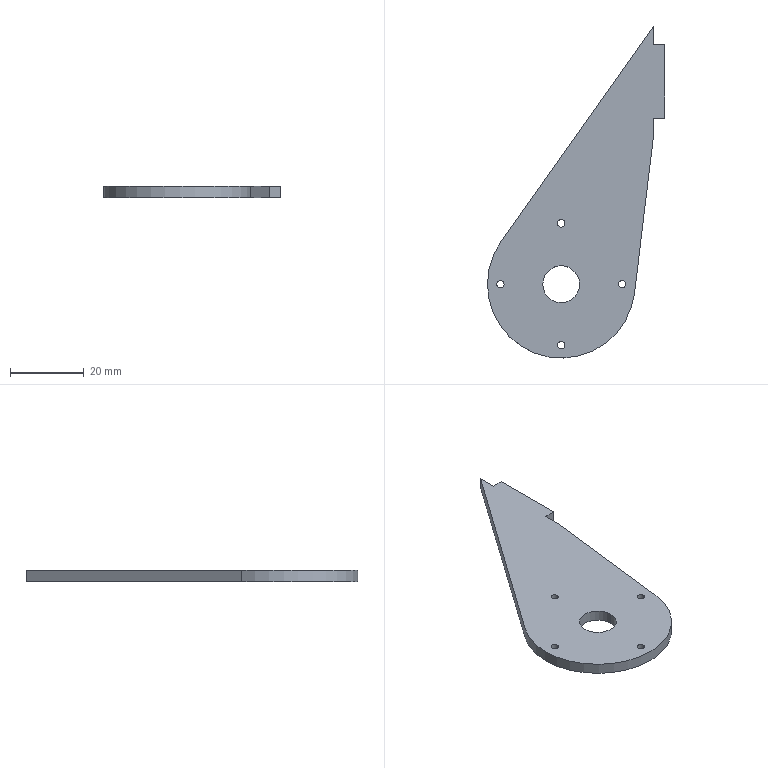Part | SolidWorks | features ICE 3, Extrusion 1 | 1 solid | 20 faces | box 48 x 90 x 3 mm | volume 6643 mm3 | cylinder 11 | plane 9 | commonest cylinder face diameters 2 x8 10 x2 40 x1
STEP:
#1=CARTESIAN_POINT('',(-17.5,0.,-3.));
#2=VERTEX_POINT('',#1);
#3=CARTESIAN_POINT('',(-15.5,0.,-3.));
#4=VERTEX_POINT('',#3);
#5=CARTESIAN_POINT('',(-16.5,0.,-3.));
#6=DIRECTION('',(0.,0.,1.));
#7=DIRECTION('',(1.,0.,0.));
#8=AXIS2_PLACEMENT_3D('',#5,#6,#7);
#9=CIRCLE('',#8,1.);
#10=EDGE_CURVE('',#2,#4,#9,.T.);
#11=ORIENTED_EDGE('',*,*,#10,.F.);
#12=CARTESIAN_POINT('',(-17.5,0.,0.));
#13=VERTEX_POINT('',#12);
#14=CARTESIAN_POINT('',(-17.5,0.,-10.));
#15=DIRECTION('',(0.,0.,1.));
#16=VECTOR('',#15,1000.);
#17=LINE('',#14,#16);
#18=EDGE_CURVE('',#2,#13,#17,.T.);
#19=ORIENTED_EDGE('',*,*,#18,.T.);
#20=CARTESIAN_POINT('',(-15.5,0.,0.));
#21=VERTEX_POINT('',#20);
#22=CARTESIAN_POINT('',(-16.5,0.,0.));
#23=DIRECTION('',(0.,0.,1.));
#24=DIRECTION('',(1.,0.,0.));
#25=AXIS2_PLACEMENT_3D('',#22,#23,#24);
#26=CIRCLE('',#25,1.);
#27=EDGE_CURVE('',#13,#21,#26,.T.);
#28=ORIENTED_EDGE('',*,*,#27,.T.);
#29=CARTESIAN_POINT('',(-15.5,0.,-10.));
#30=DIRECTION('',(0.,0.,1.));
#31=VECTOR('',#30,1000.);
#32=LINE('',#29,#31);
#33=EDGE_CURVE('',#4,#21,#32,.T.);
#34=ORIENTED_EDGE('',*,*,#33,.F.);
#35=EDGE_LOOP('',(#11,#19,#28,#34));
#36=FACE_OUTER_BOUND('',#35,.T.);
#37=CARTESIAN_POINT('',(-16.5,0.,-10.));
#38=DIRECTION('',(0.,0.,1.));
#39=DIRECTION('',(1.,0.,0.));
#40=AXIS2_PLACEMENT_3D('',#37,#38,#39);
#41=CYLINDRICAL_SURFACE('',#40,1.);
#42=ADVANCED_FACE('',(#36),#41,.F.);
#43=CARTESIAN_POINT('',(15.5,0.,-3.));
#44=VERTEX_POINT('',#43);
#45=CARTESIAN_POINT('',(17.5,0.,-3.));
#46=VERTEX_POINT('',#45);
#47=CARTESIAN_POINT('',(16.5,0.,-3.));
#48=DIRECTION('',(0.,0.,1.));
#49=DIRECTION('',(1.,0.,0.));
#50=AXIS2_PLACEMENT_3D('',#47,#48,#49);
#51=CIRCLE('',#50,1.);
#52=EDGE_CURVE('',#44,#46,#51,.T.);
#53=ORIENTED_EDGE('',*,*,#52,.F.);
#54=CARTESIAN_POINT('',(15.5,0.,0.));
#55=VERTEX_POINT('',#54);
#56=CARTESIAN_POINT('',(15.5,0.,-10.));
#57=DIRECTION('',(0.,0.,1.));
#58=VECTOR('',#57,1000.);
#59=LINE('',#56,#58);
#60=EDGE_CURVE('',#44,#55,#59,.T.);
#61=ORIENTED_EDGE('',*,*,#60,.T.);
#62=CARTESIAN_POINT('',(17.5,0.,0.));
#63=VERTEX_POINT('',#62);
#64=CARTESIAN_POINT('',(16.5,0.,0.));
#65=DIRECTION('',(0.,0.,1.));
#66=DIRECTION('',(1.,0.,0.));
#67=AXIS2_PLACEMENT_3D('',#64,#65,#66);
#68=CIRCLE('',#67,1.);
#69=EDGE_CURVE('',#55,#63,#68,.T.);
#70=ORIENTED_EDGE('',*,*,#69,.T.);
#71=CARTESIAN_POINT('',(17.5,0.,-10.));
#72=DIRECTION('',(0.,0.,1.));
#73=VECTOR('',#72,1000.);
#74=LINE('',#71,#73);
#75=EDGE_CURVE('',#46,#63,#74,.T.);
#76=ORIENTED_EDGE('',*,*,#75,.F.);
#77=EDGE_LOOP('',(#53,#61,#70,#76));
#78=FACE_OUTER_BOUND('',#77,.T.);
#79=CARTESIAN_POINT('',(16.5,0.,-10.));
#80=DIRECTION('',(0.,0.,1.));
#81=DIRECTION('',(1.,0.,0.));
#82=AXIS2_PLACEMENT_3D('',#79,#80,#81);
#83=CYLINDRICAL_SURFACE('',#82,1.);
#84=ADVANCED_FACE('',(#78),#83,.F.);
#85=CARTESIAN_POINT('',(-1.,-16.5,-3.));
#86=VERTEX_POINT('',#85);
#87=CARTESIAN_POINT('',(1.,-16.5,-3.));
#88=VERTEX_POINT('',#87);
#89=CARTESIAN_POINT('',(0.,-16.5,-3.));
#90=DIRECTION('',(0.,0.,1.));
#91=DIRECTION('',(1.,0.,0.));
#92=AXIS2_PLACEMENT_3D('',#89,#90,#91);
#93=CIRCLE('',#92,1.);
#94=EDGE_CURVE('',#86,#88,#93,.T.);
#95=ORIENTED_EDGE('',*,*,#94,.F.);
#96=CARTESIAN_POINT('',(-1.,-16.5,0.));
#97=VERTEX_POINT('',#96);
#98=CARTESIAN_POINT('',(-1.,-16.5,-10.));
#99=DIRECTION('',(0.,0.,1.));
#100=VECTOR('',#99,1000.);
#101=LINE('',#98,#100);
#102=EDGE_CURVE('',#86,#97,#101,.T.);
#103=ORIENTED_EDGE('',*,*,#102,.T.);
#104=CARTESIAN_POINT('',(1.,-16.5,0.));
#105=VERTEX_POINT('',#104);
#106=CARTESIAN_POINT('',(0.,-16.5,0.));
#107=DIRECTION('',(0.,0.,1.));
#108=DIRECTION('',(1.,0.,0.));
#109=AXIS2_PLACEMENT_3D('',#106,#107,#108);
#110=CIRCLE('',#109,1.);
#111=EDGE_CURVE('',#97,#105,#110,.T.);
#112=ORIENTED_EDGE('',*,*,#111,.T.);
#113=CARTESIAN_POINT('',(1.,-16.5,-10.));
#114=DIRECTION('',(0.,0.,1.));
#115=VECTOR('',#114,1000.);
#116=LINE('',#113,#115);
#117=EDGE_CURVE('',#88,#105,#116,.T.);
#118=ORIENTED_EDGE('',*,*,#117,.F.);
#119=EDGE_LOOP('',(#95,#103,#112,#118));
#120=FACE_OUTER_BOUND('',#119,.T.);
#121=CARTESIAN_POINT('',(0.,-16.5,-10.));
#122=DIRECTION('',(0.,0.,1.));
#123=DIRECTION('',(1.,0.,0.));
#124=AXIS2_PLACEMENT_3D('',#121,#122,#123);
#125=CYLINDRICAL_SURFACE('',#124,1.);
#126=ADVANCED_FACE('',(#120),#125,.F.);
#127=CARTESIAN_POINT('',(-1.,16.5,-3.));
#128=VERTEX_POINT('',#127);
#129=CARTESIAN_POINT('',(1.,16.5,-3.));
#130=VERTEX_POINT('',#129);
#131=CARTESIAN_POINT('',(0.,16.5,-3.));
#132=DIRECTION('',(0.,0.,1.));
#133=DIRECTION('',(1.,0.,0.));
#134=AXIS2_PLACEMENT_3D('',#131,#132,#133);
#135=CIRCLE('',#134,1.);
#136=EDGE_CURVE('',#128,#130,#135,.T.);
#137=ORIENTED_EDGE('',*,*,#136,.F.);
#138=CARTESIAN_POINT('',(-1.,16.5,0.));
#139=VERTEX_POINT('',#138);
#140=CARTESIAN_POINT('',(-1.,16.5,-10.));
#141=DIRECTION('',(0.,0.,1.));
#142=VECTOR('',#141,1000.);
#143=LINE('',#140,#142);
#144=EDGE_CURVE('',#128,#139,#143,.T.);
#145=ORIENTED_EDGE('',*,*,#144,.T.);
#146=CARTESIAN_POINT('',(1.,16.5,0.));
#147=VERTEX_POINT('',#146);
#148=CARTESIAN_POINT('',(0.,16.5,0.));
#149=DIRECTION('',(0.,0.,1.));
#150=DIRECTION('',(1.,0.,0.));
#151=AXIS2_PLACEMENT_3D('',#148,#149,#150);
#152=CIRCLE('',#151,1.);
#153=EDGE_CURVE('',#139,#147,#152,.T.);
#154=ORIENTED_EDGE('',*,*,#153,.T.);
#155=CARTESIAN_POINT('',(1.,16.5,-10.));
#156=DIRECTION('',(0.,0.,1.));
#157=VECTOR('',#156,1000.);
#158=LINE('',#155,#157);
#159=EDGE_CURVE('',#130,#147,#158,.T.);
#160=ORIENTED_EDGE('',*,*,#159,.F.);
#161=EDGE_LOOP('',(#137,#145,#154,#160));
#162=FACE_OUTER_BOUND('',#161,.T.);
#163=CARTESIAN_POINT('',(0.,16.5,-10.));
#164=DIRECTION('',(0.,0.,1.));
#165=DIRECTION('',(1.,0.,0.));
#166=AXIS2_PLACEMENT_3D('',#163,#164,#165);
#167=CYLINDRICAL_SURFACE('',#166,1.);
#168=ADVANCED_FACE('',(#162),#167,.F.);
#169=CARTESIAN_POINT('',(-5.,0.,-3.));
#170=VERTEX_POINT('',#169);
#171=CARTESIAN_POINT('',(5.,0.,-3.));
#172=VERTEX_POINT('',#171);
#173=CARTESIAN_POINT('',(0.,0.,-3.));
#174=DIRECTION('',(0.,0.,1.));
#175=DIRECTION('',(1.,0.,0.));
#176=AXIS2_PLACEMENT_3D('',#173,#174,#175);
#177=CIRCLE('',#176,5.);
#178=EDGE_CURVE('',#170,#172,#177,.T.);
#179=ORIENTED_EDGE('',*,*,#178,.F.);
#180=CARTESIAN_POINT('',(-5.,0.,0.));
#181=VERTEX_POINT('',#180);
#182=CARTESIAN_POINT('',(-5.,0.,-10.));
#183=DIRECTION('',(0.,0.,1.));
#184=VECTOR('',#183,1000.);
#185=LINE('',#182,#184);
#186=EDGE_CURVE('',#170,#181,#185,.T.);
#187=ORIENTED_EDGE('',*,*,#186,.T.);
#188=CARTESIAN_POINT('',(5.,0.,0.));
#189=VERTEX_POINT('',#188);
#190=CARTESIAN_POINT('',(0.,0.,0.));
#191=DIRECTION('',(0.,0.,1.));
#192=DIRECTION('',(1.,0.,0.));
#193=AXIS2_PLACEMENT_3D('',#190,#191,#192);
#194=CIRCLE('',#193,5.);
#195=EDGE_CURVE('',#181,#189,#194,.T.);
#196=ORIENTED_EDGE('',*,*,#195,.T.);
#197=CARTESIAN_POINT('',(5.,0.,-10.));
#198=DIRECTION('',(0.,0.,1.));
#199=VECTOR('',#198,1000.);
#200=LINE('',#197,#199);
#201=EDGE_CURVE('',#172,#189,#200,.T.);
#202=ORIENTED_EDGE('',*,*,#201,.F.);
#203=EDGE_LOOP('',(#179,#187,#196,#202));
#204=FACE_OUTER_BOUND('',#203,.T.);
#205=CARTESIAN_POINT('',(0.,0.,-10.));
#206=DIRECTION('',(0.,0.,1.));
#207=DIRECTION('',(1.,0.,0.));
#208=AXIS2_PLACEMENT_3D('',#205,#206,#207);
#209=CYLINDRICAL_SURFACE('',#208,5.);
#210=ADVANCED_FACE('',(#204),#209,.F.);
#211=CARTESIAN_POINT('',(25.,65.,-3.));
#212=VERTEX_POINT('',#211);
#213=CARTESIAN_POINT('',(25.,65.,0.));
#214=VERTEX_POINT('',#213);
#215=CARTESIAN_POINT('',(25.,65.,0.));
#216=DIRECTION('',(0.,0.,1.));
#217=VECTOR('',#216,1000.);
#218=LINE('',#215,#217);
#219=EDGE_CURVE('',#212,#214,#218,.T.);
#220=ORIENTED_EDGE('',*,*,#219,.F.);
#221=CARTESIAN_POINT('',(25.,70.,-3.));
#222=VERTEX_POINT('',#221);
#223=CARTESIAN_POINT('',(25.,70.,-3.));
#224=DIRECTION('',(0.,1.,0.));
#225=VECTOR('',#224,1000.);
#226=LINE('',#223,#225);
#227=EDGE_CURVE('',#212,#222,#226,.T.);
#228=ORIENTED_EDGE('',*,*,#227,.T.);
#229=CARTESIAN_POINT('',(25.,70.,0.));
#230=VERTEX_POINT('',#229);
#231=CARTESIAN_POINT('',(25.,70.,-3.));
#232=DIRECTION('',(0.,0.,1.));
#233=VECTOR('',#232,1000.);
#234=LINE('',#231,#233);
#235=EDGE_CURVE('',#222,#230,#234,.T.);
#236=ORIENTED_EDGE('',*,*,#235,.T.);
#237=CARTESIAN_POINT('',(25.,70.,0.));
#238=DIRECTION('',(0.,1.,0.));
#239=VECTOR('',#238,1000.);
#240=LINE('',#237,#239);
#241=EDGE_CURVE('',#214,#230,#240,.T.);
#242=ORIENTED_EDGE('',*,*,#241,.F.);
#243=EDGE_LOOP('',(#220,#228,#236,#242));
#244=FACE_OUTER_BOUND('',#243,.T.);
#245=CARTESIAN_POINT('',(25.,70.,-3.));
#246=DIRECTION('',(1.,0.,0.));
#247=DIRECTION('',(0.,1.,0.));
#248=AXIS2_PLACEMENT_3D('',#245,#246,#247);
#249=PLANE('',#248);
#250=ADVANCED_FACE('',(#244),#249,.T.);
#251=CARTESIAN_POINT('',(-16.33,11.547,0.));
#252=VERTEX_POINT('',#251);
#253=CARTESIAN_POINT('',(19.854,-2.409,0.));
#254=VERTEX_POINT('',#253);
#255=CARTESIAN_POINT('',(0.,0.,0.));
#256=DIRECTION('',(0.,0.,1.));
#257=DIRECTION('',(1.,0.,0.));
#258=AXIS2_PLACEMENT_3D('',#255,#256,#257);
#259=CIRCLE('',#258,20.);
#260=EDGE_CURVE('',#252,#254,#259,.T.);
#261=ORIENTED_EDGE('',*,*,#260,.F.);
#262=CARTESIAN_POINT('',(-16.33,11.547,-3.));
#263=VERTEX_POINT('',#262);
#264=CARTESIAN_POINT('',(-16.33,11.547,-3.));
#265=DIRECTION('',(0.,0.,1.));
#266=VECTOR('',#265,1000.);
#267=LINE('',#264,#266);
#268=EDGE_CURVE('',#263,#252,#267,.T.);
#269=ORIENTED_EDGE('',*,*,#268,.F.);
#270=CARTESIAN_POINT('',(19.854,-2.409,-3.));
#271=VERTEX_POINT('',#270);
#272=CARTESIAN_POINT('',(0.,0.,-3.));
#273=DIRECTION('',(0.,0.,1.));
#274=DIRECTION('',(1.,0.,0.));
#275=AXIS2_PLACEMENT_3D('',#272,#273,#274);
#276=CIRCLE('',#275,20.);
#277=EDGE_CURVE('',#263,#271,#276,.T.);
#278=ORIENTED_EDGE('',*,*,#277,.T.);
#279=CARTESIAN_POINT('',(19.854,-2.409,-3.));
#280=DIRECTION('',(0.,0.,1.));
#281=VECTOR('',#280,1000.);
#282=LINE('',#279,#281);
#283=EDGE_CURVE('',#271,#254,#282,.T.);
#284=ORIENTED_EDGE('',*,*,#283,.T.);
#285=EDGE_LOOP('',(#261,#269,#278,#284));
#286=FACE_OUTER_BOUND('',#285,.T.);
#287=CARTESIAN_POINT('',(0.,0.,-3.));
#288=DIRECTION('',(0.,0.,1.));
#289=DIRECTION('',(1.,0.,0.));
#290=AXIS2_PLACEMENT_3D('',#287,#288,#289);
#291=CYLINDRICAL_SURFACE('',#290,20.);
#292=ADVANCED_FACE('',(#286),#291,.T.);
#293=CARTESIAN_POINT('',(-16.33,11.547,0.));
#294=DIRECTION('',(-0.5773,-0.8165,0.));
#295=VECTOR('',#294,1000.);
#296=LINE('',#293,#295);
#297=EDGE_CURVE('',#230,#252,#296,.T.);
#298=ORIENTED_EDGE('',*,*,#297,.F.);
#299=ORIENTED_EDGE('',*,*,#235,.F.);
#300=CARTESIAN_POINT('',(-16.33,11.547,-3.));
#301=DIRECTION('',(-0.5773,-0.8165,0.));
#302=VECTOR('',#301,1000.);
#303=LINE('',#300,#302);
#304=EDGE_CURVE('',#222,#263,#303,.T.);
#305=ORIENTED_EDGE('',*,*,#304,.T.);
#306=ORIENTED_EDGE('',*,*,#268,.T.);
#307=EDGE_LOOP('',(#298,#299,#305,#306));
#308=FACE_OUTER_BOUND('',#307,.T.);
#309=CARTESIAN_POINT('',(-16.33,11.547,-3.));
#310=DIRECTION('',(-0.8165,0.5773,0.));
#311=DIRECTION('',(-0.5773,-0.8165,0.));
#312=AXIS2_PLACEMENT_3D('',#309,#310,#311);
#313=PLANE('',#312);
#314=ADVANCED_FACE('',(#308),#313,.T.);
#315=CARTESIAN_POINT('',(25.,45.,0.));
#316=VERTEX_POINT('',#315);
#317=CARTESIAN_POINT('',(25.,45.,-3.));
#318=VERTEX_POINT('',#317);
#319=CARTESIAN_POINT('',(25.,45.,0.));
#320=DIRECTION('',(0.,0.,-1.));
#321=VECTOR('',#320,1000.);
#322=LINE('',#319,#321);
#323=EDGE_CURVE('',#316,#318,#322,.T.);
#324=ORIENTED_EDGE('',*,*,#323,.F.);
#325=CARTESIAN_POINT('',(25.,40.,0.));
#326=VERTEX_POINT('',#325);
#327=CARTESIAN_POINT('',(25.,70.,0.));
#328=DIRECTION('',(0.,1.,0.));
#329=VECTOR('',#328,1000.);
#330=LINE('',#327,#329);
#331=EDGE_CURVE('',#326,#316,#330,.T.);
#332=ORIENTED_EDGE('',*,*,#331,.F.);
#333=CARTESIAN_POINT('',(25.,40.,-3.));
#334=VERTEX_POINT('',#333);
#335=CARTESIAN_POINT('',(25.,40.,-3.));
#336=DIRECTION('',(0.,0.,1.));
#337=VECTOR('',#336,1000.);
#338=LINE('',#335,#337);
#339=EDGE_CURVE('',#334,#326,#338,.T.);
#340=ORIENTED_EDGE('',*,*,#339,.F.);
#341=CARTESIAN_POINT('',(25.,70.,-3.));
#342=DIRECTION('',(0.,1.,0.));
#343=VECTOR('',#342,1000.);
#344=LINE('',#341,#343);
#345=EDGE_CURVE('',#334,#318,#344,.T.);
#346=ORIENTED_EDGE('',*,*,#345,.T.);
#347=EDGE_LOOP('',(#324,#332,#340,#346));
#348=FACE_OUTER_BOUND('',#347,.T.);
#349=CARTESIAN_POINT('',(25.,70.,-3.));
#350=DIRECTION('',(1.,0.,0.));
#351=DIRECTION('',(0.,1.,0.));
#352=AXIS2_PLACEMENT_3D('',#349,#350,#351);
#353=PLANE('',#352);
#354=ADVANCED_FACE('',(#348),#353,.T.);
#355=CARTESIAN_POINT('',(25.,40.,0.));
#356=DIRECTION('',(0.1204,0.9927,0.));
#357=VECTOR('',#356,1000.);
#358=LINE('',#355,#357);
#359=EDGE_CURVE('',#254,#326,#358,.T.);
#360=ORIENTED_EDGE('',*,*,#359,.F.);
#361=ORIENTED_EDGE('',*,*,#283,.F.);
#362=CARTESIAN_POINT('',(25.,40.,-3.));
#363=DIRECTION('',(0.1204,0.9927,0.));
#364=VECTOR('',#363,1000.);
#365=LINE('',#362,#364);
#366=EDGE_CURVE('',#271,#334,#365,.T.);
#367=ORIENTED_EDGE('',*,*,#366,.T.);
#368=ORIENTED_EDGE('',*,*,#339,.T.);
#369=EDGE_LOOP('',(#360,#361,#367,#368));
#370=FACE_OUTER_BOUND('',#369,.T.);
#371=CARTESIAN_POINT('',(25.,40.,-3.));
#372=DIRECTION('',(0.9927,-0.1204,0.));
#373=DIRECTION('',(0.1204,0.9927,0.));
#374=AXIS2_PLACEMENT_3D('',#371,#372,#373);
#375=PLANE('',#374);
#376=ADVANCED_FACE('',(#370),#375,.T.);
#377=CARTESIAN_POINT('',(-16.5,0.,-3.));
#378=DIRECTION('',(0.,0.,1.));
#379=DIRECTION('',(1.,0.,0.));
#380=AXIS2_PLACEMENT_3D('',#377,#378,#379);
#381=CIRCLE('',#380,1.);
#382=EDGE_CURVE('',#4,#2,#381,.T.);
#383=ORIENTED_EDGE('',*,*,#382,.T.);
#384=ORIENTED_EDGE('',*,*,#10,.T.);
#385=EDGE_LOOP('',(#383,#384));
#386=FACE_BOUND('',#385,.T.);
#387=CARTESIAN_POINT('',(16.5,0.,-3.));
#388=DIRECTION('',(0.,0.,1.));
#389=DIRECTION('',(1.,0.,0.));
#390=AXIS2_PLACEMENT_3D('',#387,#388,#389);
#391=CIRCLE('',#390,1.);
#392=EDGE_CURVE('',#46,#44,#391,.T.);
#393=ORIENTED_EDGE('',*,*,#392,.T.);
#394=ORIENTED_EDGE('',*,*,#52,.T.);
#395=EDGE_LOOP('',(#393,#394));
#396=FACE_BOUND('',#395,.T.);
#397=CARTESIAN_POINT('',(0.,-16.5,-3.));
#398=DIRECTION('',(0.,0.,1.));
#399=DIRECTION('',(1.,0.,0.));
#400=AXIS2_PLACEMENT_3D('',#397,#398,#399);
#401=CIRCLE('',#400,1.);
#402=EDGE_CURVE('',#88,#86,#401,.T.);
#403=ORIENTED_EDGE('',*,*,#402,.T.);
#404=ORIENTED_EDGE('',*,*,#94,.T.);
#405=EDGE_LOOP('',(#403,#404));
#406=FACE_BOUND('',#405,.T.);
#407=CARTESIAN_POINT('',(0.,16.5,-3.));
#408=DIRECTION('',(0.,0.,1.));
#409=DIRECTION('',(1.,0.,0.));
#410=AXIS2_PLACEMENT_3D('',#407,#408,#409);
#411=CIRCLE('',#410,1.);
#412=EDGE_CURVE('',#130,#128,#411,.T.);
#413=ORIENTED_EDGE('',*,*,#412,.T.);
#414=ORIENTED_EDGE('',*,*,#136,.T.);
#415=EDGE_LOOP('',(#413,#414));
#416=FACE_BOUND('',#415,.T.);
#417=CARTESIAN_POINT('',(0.,0.,-3.));
#418=DIRECTION('',(0.,0.,1.));
#419=DIRECTION('',(1.,0.,0.));
#420=AXIS2_PLACEMENT_3D('',#417,#418,#419);
#421=CIRCLE('',#420,5.);
#422=EDGE_CURVE('',#172,#170,#421,.T.);
#423=ORIENTED_EDGE('',*,*,#422,.T.);
#424=ORIENTED_EDGE('',*,*,#178,.T.);
#425=EDGE_LOOP('',(#423,#424));
#426=FACE_BOUND('',#425,.T.);
#427=ORIENTED_EDGE('',*,*,#277,.F.);
#428=ORIENTED_EDGE('',*,*,#304,.F.);
#429=ORIENTED_EDGE('',*,*,#227,.F.);
#430=CARTESIAN_POINT('',(28.,65.,-3.));
#431=VERTEX_POINT('',#430);
#432=CARTESIAN_POINT('',(28.,65.,-3.));
#433=DIRECTION('',(-1.,0.,0.));
#434=VECTOR('',#433,1000.);
#435=LINE('',#432,#434);
#436=EDGE_CURVE('',#431,#212,#435,.T.);
#437=ORIENTED_EDGE('',*,*,#436,.F.);
#438=CARTESIAN_POINT('',(28.,45.,-3.));
#439=VERTEX_POINT('',#438);
#440=CARTESIAN_POINT('',(28.,65.,-3.));
#441=DIRECTION('',(0.,1.,0.));
#442=VECTOR('',#441,1000.);
#443=LINE('',#440,#442);
#444=EDGE_CURVE('',#439,#431,#443,.T.);
#445=ORIENTED_EDGE('',*,*,#444,.F.);
#446=CARTESIAN_POINT('',(28.,45.,-3.));
#447=DIRECTION('',(-1.,0.,0.));
#448=VECTOR('',#447,1000.);
#449=LINE('',#446,#448);
#450=EDGE_CURVE('',#439,#318,#449,.T.);
#451=ORIENTED_EDGE('',*,*,#450,.T.);
#452=ORIENTED_EDGE('',*,*,#345,.F.);
#453=ORIENTED_EDGE('',*,*,#366,.F.);
#454=EDGE_LOOP('',(#427,#428,#429,#437,#445,#451,#452,#453));
#455=FACE_OUTER_BOUND('',#454,.T.);
#456=CARTESIAN_POINT('',(0.,0.,-3.));
#457=DIRECTION('',(0.,0.,1.));
#458=DIRECTION('',(1.,0.,0.));
#459=AXIS2_PLACEMENT_3D('',#456,#457,#458);
#460=PLANE('',#459);
#461=ADVANCED_FACE('',(#386,#396,#406,#416,#426,#455),#460,.F.);
#462=CARTESIAN_POINT('',(-16.5,0.,0.));
#463=DIRECTION('',(0.,0.,1.));
#464=DIRECTION('',(1.,0.,0.));
#465=AXIS2_PLACEMENT_3D('',#462,#463,#464);
#466=CIRCLE('',#465,1.);
#467=EDGE_CURVE('',#21,#13,#466,.T.);
#468=ORIENTED_EDGE('',*,*,#467,.F.);
#469=ORIENTED_EDGE('',*,*,#27,.F.);
#470=EDGE_LOOP('',(#468,#469));
#471=FACE_BOUND('',#470,.T.);
#472=CARTESIAN_POINT('',(16.5,0.,0.));
#473=DIRECTION('',(0.,0.,1.));
#474=DIRECTION('',(1.,0.,0.));
#475=AXIS2_PLACEMENT_3D('',#472,#473,#474);
#476=CIRCLE('',#475,1.);
#477=EDGE_CURVE('',#63,#55,#476,.T.);
#478=ORIENTED_EDGE('',*,*,#477,.F.);
#479=ORIENTED_EDGE('',*,*,#69,.F.);
#480=EDGE_LOOP('',(#478,#479));
#481=FACE_BOUND('',#480,.T.);
#482=CARTESIAN_POINT('',(0.,-16.5,0.));
#483=DIRECTION('',(0.,0.,1.));
#484=DIRECTION('',(1.,0.,0.));
#485=AXIS2_PLACEMENT_3D('',#482,#483,#484);
#486=CIRCLE('',#485,1.);
#487=EDGE_CURVE('',#105,#97,#486,.T.);
#488=ORIENTED_EDGE('',*,*,#487,.F.);
#489=ORIENTED_EDGE('',*,*,#111,.F.);
#490=EDGE_LOOP('',(#488,#489));
#491=FACE_BOUND('',#490,.T.);
#492=CARTESIAN_POINT('',(0.,16.5,0.));
#493=DIRECTION('',(0.,0.,1.));
#494=DIRECTION('',(1.,0.,0.));
#495=AXIS2_PLACEMENT_3D('',#492,#493,#494);
#496=CIRCLE('',#495,1.);
#497=EDGE_CURVE('',#147,#139,#496,.T.);
#498=ORIENTED_EDGE('',*,*,#497,.F.);
#499=ORIENTED_EDGE('',*,*,#153,.F.);
#500=EDGE_LOOP('',(#498,#499));
#501=FACE_BOUND('',#500,.T.);
#502=CARTESIAN_POINT('',(0.,0.,0.));
#503=DIRECTION('',(0.,0.,1.));
#504=DIRECTION('',(1.,0.,0.));
#505=AXIS2_PLACEMENT_3D('',#502,#503,#504);
#506=CIRCLE('',#505,5.);
#507=EDGE_CURVE('',#189,#181,#506,.T.);
#508=ORIENTED_EDGE('',*,*,#507,.F.);
#509=ORIENTED_EDGE('',*,*,#195,.F.);
#510=EDGE_LOOP('',(#508,#509));
#511=FACE_BOUND('',#510,.T.);
#512=ORIENTED_EDGE('',*,*,#260,.T.);
#513=ORIENTED_EDGE('',*,*,#359,.T.);
#514=ORIENTED_EDGE('',*,*,#331,.T.);
#515=CARTESIAN_POINT('',(28.,45.,0.));
#516=VERTEX_POINT('',#515);
#517=CARTESIAN_POINT('',(28.,45.,0.));
#518=DIRECTION('',(-1.,0.,0.));
#519=VECTOR('',#518,1000.);
#520=LINE('',#517,#519);
#521=EDGE_CURVE('',#516,#316,#520,.T.);
#522=ORIENTED_EDGE('',*,*,#521,.F.);
#523=CARTESIAN_POINT('',(28.,65.,0.));
#524=VERTEX_POINT('',#523);
#525=CARTESIAN_POINT('',(28.,65.,0.));
#526=DIRECTION('',(0.,-1.,0.));
#527=VECTOR('',#526,1000.);
#528=LINE('',#525,#527);
#529=EDGE_CURVE('',#524,#516,#528,.T.);
#530=ORIENTED_EDGE('',*,*,#529,.F.);
#531=CARTESIAN_POINT('',(28.,65.,0.));
#532=DIRECTION('',(-1.,0.,0.));
#533=VECTOR('',#532,1000.);
#534=LINE('',#531,#533);
#535=EDGE_CURVE('',#524,#214,#534,.T.);
#536=ORIENTED_EDGE('',*,*,#535,.T.);
#537=ORIENTED_EDGE('',*,*,#241,.T.);
#538=ORIENTED_EDGE('',*,*,#297,.T.);
#539=EDGE_LOOP('',(#512,#513,#514,#522,#530,#536,#537,#538));
#540=FACE_OUTER_BOUND('',#539,.T.);
#541=CARTESIAN_POINT('',(0.,0.,0.));
#542=DIRECTION('',(0.,0.,1.));
#543=DIRECTION('',(1.,0.,0.));
#544=AXIS2_PLACEMENT_3D('',#541,#542,#543);
#545=PLANE('',#544);
#546=ADVANCED_FACE('',(#471,#481,#491,#501,#511,#540),#545,.T.);
#547=ORIENTED_EDGE('',*,*,#186,.F.);
#548=ORIENTED_EDGE('',*,*,#422,.F.);
#549=ORIENTED_EDGE('',*,*,#201,.T.);
#550=ORIENTED_EDGE('',*,*,#507,.T.);
#551=EDGE_LOOP('',(#547,#548,#549,#550));
#552=FACE_OUTER_BOUND('',#551,.T.);
#553=CARTESIAN_POINT('',(0.,0.,-10.));
#554=DIRECTION('',(0.,0.,1.));
#555=DIRECTION('',(1.,0.,0.));
#556=AXIS2_PLACEMENT_3D('',#553,#554,#555);
#557=CYLINDRICAL_SURFACE('',#556,5.);
#558=ADVANCED_FACE('',(#552),#557,.F.);
#559=ORIENTED_EDGE('',*,*,#323,.T.);
#560=ORIENTED_EDGE('',*,*,#450,.F.);
#561=CARTESIAN_POINT('',(28.,45.,0.));
#562=DIRECTION('',(0.,0.,-1.));
#563=VECTOR('',#562,1000.);
#564=LINE('',#561,#563);
#565=EDGE_CURVE('',#516,#439,#564,.T.);
#566=ORIENTED_EDGE('',*,*,#565,.F.);
#567=ORIENTED_EDGE('',*,*,#521,.T.);
#568=EDGE_LOOP('',(#559,#560,#566,#567));
#569=FACE_OUTER_BOUND('',#568,.T.);
#570=CARTESIAN_POINT('',(28.,45.,0.));
#571=DIRECTION('',(0.,1.,0.));
#572=DIRECTION('',(-1.,0.,0.));
#573=AXIS2_PLACEMENT_3D('',#570,#571,#572);
#574=PLANE('',#573);
#575=ADVANCED_FACE('',(#569),#574,.F.);
#576=ORIENTED_EDGE('',*,*,#219,.T.);
#577=ORIENTED_EDGE('',*,*,#535,.F.);
#578=CARTESIAN_POINT('',(28.,65.,0.));
#579=DIRECTION('',(0.,0.,1.));
#580=VECTOR('',#579,1000.);
#581=LINE('',#578,#580);
#582=EDGE_CURVE('',#431,#524,#581,.T.);
#583=ORIENTED_EDGE('',*,*,#582,.F.);
#584=ORIENTED_EDGE('',*,*,#436,.T.);
#585=EDGE_LOOP('',(#576,#577,#583,#584));
#586=FACE_OUTER_BOUND('',#585,.T.);
#587=CARTESIAN_POINT('',(28.,65.,0.));
#588=DIRECTION('',(0.,-1.,0.));
#589=DIRECTION('',(1.,0.,0.));
#590=AXIS2_PLACEMENT_3D('',#587,#588,#589);
#591=PLANE('',#590);
#592=ADVANCED_FACE('',(#586),#591,.F.);
#593=ORIENTED_EDGE('',*,*,#529,.T.);
#594=ORIENTED_EDGE('',*,*,#565,.T.);
#595=ORIENTED_EDGE('',*,*,#444,.T.);
#596=ORIENTED_EDGE('',*,*,#582,.T.);
#597=EDGE_LOOP('',(#593,#594,#595,#596));
#598=FACE_OUTER_BOUND('',#597,.T.);
#599=CARTESIAN_POINT('',(28.,0.,0.));
#600=DIRECTION('',(1.,0.,0.));
#601=DIRECTION('',(0.,1.,0.));
#602=AXIS2_PLACEMENT_3D('',#599,#600,#601);
#603=PLANE('',#602);
#604=ADVANCED_FACE('',(#598),#603,.T.);
#605=ORIENTED_EDGE('',*,*,#144,.F.);
#606=ORIENTED_EDGE('',*,*,#412,.F.);
#607=ORIENTED_EDGE('',*,*,#159,.T.);
#608=ORIENTED_EDGE('',*,*,#497,.T.);
#609=EDGE_LOOP('',(#605,#606,#607,#608));
#610=FACE_OUTER_BOUND('',#609,.T.);
#611=CARTESIAN_POINT('',(0.,16.5,-10.));
#612=DIRECTION('',(0.,0.,1.));
#613=DIRECTION('',(1.,0.,0.));
#614=AXIS2_PLACEMENT_3D('',#611,#612,#613);
#615=CYLINDRICAL_SURFACE('',#614,1.);
#616=ADVANCED_FACE('',(#610),#615,.F.);
#617=ORIENTED_EDGE('',*,*,#102,.F.);
#618=ORIENTED_EDGE('',*,*,#402,.F.);
#619=ORIENTED_EDGE('',*,*,#117,.T.);
#620=ORIENTED_EDGE('',*,*,#487,.T.);
#621=EDGE_LOOP('',(#617,#618,#619,#620));
#622=FACE_OUTER_BOUND('',#621,.T.);
#623=CARTESIAN_POINT('',(0.,-16.5,-10.));
#624=DIRECTION('',(0.,0.,1.));
#625=DIRECTION('',(1.,0.,0.));
#626=AXIS2_PLACEMENT_3D('',#623,#624,#625);
#627=CYLINDRICAL_SURFACE('',#626,1.);
#628=ADVANCED_FACE('',(#622),#627,.F.);
#629=ORIENTED_EDGE('',*,*,#60,.F.);
#630=ORIENTED_EDGE('',*,*,#392,.F.);
#631=ORIENTED_EDGE('',*,*,#75,.T.);
#632=ORIENTED_EDGE('',*,*,#477,.T.);
#633=EDGE_LOOP('',(#629,#630,#631,#632));
#634=FACE_OUTER_BOUND('',#633,.T.);
#635=CARTESIAN_POINT('',(16.5,0.,-10.));
#636=DIRECTION('',(0.,0.,1.));
#637=DIRECTION('',(1.,0.,0.));
#638=AXIS2_PLACEMENT_3D('',#635,#636,#637);
#639=CYLINDRICAL_SURFACE('',#638,1.);
#640=ADVANCED_FACE('',(#634),#639,.F.);
#641=ORIENTED_EDGE('',*,*,#18,.F.);
#642=ORIENTED_EDGE('',*,*,#382,.F.);
#643=ORIENTED_EDGE('',*,*,#33,.T.);
#644=ORIENTED_EDGE('',*,*,#467,.T.);
#645=EDGE_LOOP('',(#641,#642,#643,#644));
#646=FACE_OUTER_BOUND('',#645,.T.);
#647=CARTESIAN_POINT('',(-16.5,0.,-10.));
#648=DIRECTION('',(0.,0.,1.));
#649=DIRECTION('',(1.,0.,0.));
#650=AXIS2_PLACEMENT_3D('',#647,#648,#649);
#651=CYLINDRICAL_SURFACE('',#650,1.);
#652=ADVANCED_FACE('',(#646),#651,.F.);
#653=CLOSED_SHELL('',(#42,#84,#126,#168,#210,#250,#292,#314,#354,#376,#461,#546,#558,#575,#592,#604,#616,#628,#640,#652));
#654=MANIFOLD_SOLID_BREP('',#653);
#655=CARTESIAN_POINT('',(0.,0.,0.));
#656=DIRECTION('',(0.,0.,1.));
#657=DIRECTION('',(1.,0.,0.));
#658=AXIS2_PLACEMENT_3D('',#655,#656,#657);
#659=(LENGTH_UNIT()NAMED_UNIT(*)SI_UNIT(.MILLI.,.METRE.));
#660=UNCERTAINTY_MEASURE_WITH_UNIT(LENGTH_MEASURE(0.00001),#659,'','');
#661=(NAMED_UNIT(*)PLANE_ANGLE_UNIT()SI_UNIT($,.RADIAN.));
#662=(NAMED_UNIT(*)SI_UNIT($,.STERADIAN.)SOLID_ANGLE_UNIT());
#663=(GEOMETRIC_REPRESENTATION_CONTEXT(3)GLOBAL_UNCERTAINTY_ASSIGNED_CONTEXT((#660))GLOBAL_UNIT_ASSIGNED_CONTEXT((#659,#661,#662))REPRESENTATION_CONTEXT('',''));
#664=ADVANCED_BREP_SHAPE_REPRESENTATION('',(#654,#658),#663);